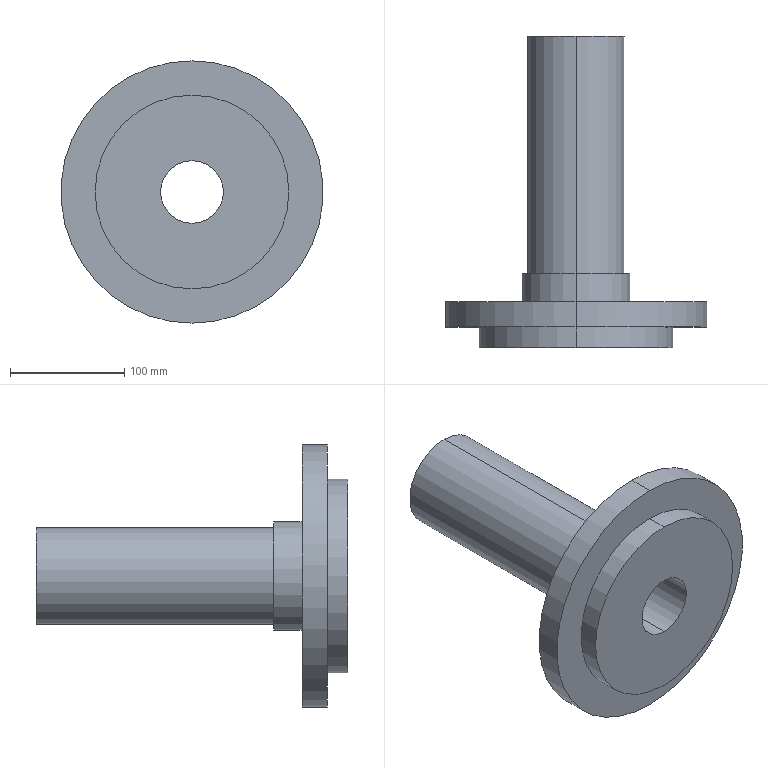Part | SolidWorks | features BaseBody 1 | 1 solid | 15 faces | box 230 x 273 x 230 mm | volume 2031428 mm3 | cylinder 10 | plane 5 | commonest cylinder face diameters 55 x2 84.997 x2 95 x2 170 x2 230 x2
STEP:
#1=CARTESIAN_POINT('',(0.,255.,27.5));
#2=VERTEX_POINT('',#1);
#3=CARTESIAN_POINT('',(0.,255.,-27.5));
#4=VERTEX_POINT('',#3);
#5=CARTESIAN_POINT('',(0.,255.,0.));
#6=DIRECTION('',(0.,-1.,0.));
#7=DIRECTION('',(0.,0.,-1.));
#8=AXIS2_PLACEMENT_3D('',#5,#6,#7);
#9=CIRCLE('',#8,27.5);
#10=EDGE_CURVE('',#2,#4,#9,.T.);
#11=ORIENTED_EDGE('',*,*,#10,.F.);
#12=CARTESIAN_POINT('',(0.,-18.,27.5));
#13=VERTEX_POINT('',#12);
#14=CARTESIAN_POINT('',(0.,255.,27.5));
#15=DIRECTION('',(0.,-1.,0.));
#16=VECTOR('',#15,1000.);
#17=LINE('',#14,#16);
#18=EDGE_CURVE('',#2,#13,#17,.T.);
#19=ORIENTED_EDGE('',*,*,#18,.T.);
#20=CARTESIAN_POINT('',(0.,-18.,-27.5));
#21=VERTEX_POINT('',#20);
#22=CARTESIAN_POINT('',(0.,-18.,0.));
#23=DIRECTION('',(0.,-1.,0.));
#24=DIRECTION('',(0.,0.,-1.));
#25=AXIS2_PLACEMENT_3D('',#22,#23,#24);
#26=CIRCLE('',#25,27.5);
#27=EDGE_CURVE('',#13,#21,#26,.T.);
#28=ORIENTED_EDGE('',*,*,#27,.T.);
#29=CARTESIAN_POINT('',(0.,255.,-27.5));
#30=DIRECTION('',(0.,-1.,0.));
#31=VECTOR('',#30,1000.);
#32=LINE('',#29,#31);
#33=EDGE_CURVE('',#4,#21,#32,.T.);
#34=ORIENTED_EDGE('',*,*,#33,.F.);
#35=EDGE_LOOP('',(#11,#19,#28,#34));
#36=FACE_OUTER_BOUND('',#35,.T.);
#37=CARTESIAN_POINT('',(0.,255.,0.));
#38=DIRECTION('',(0.,-1.,0.));
#39=DIRECTION('',(0.,0.,-1.));
#40=AXIS2_PLACEMENT_3D('',#37,#38,#39);
#41=CYLINDRICAL_SURFACE('',#40,27.5);
#42=ADVANCED_FACE('',(#36),#41,.F.);
#43=CARTESIAN_POINT('',(0.,255.,42.498));
#44=VERTEX_POINT('',#43);
#45=CARTESIAN_POINT('',(0.,255.,-42.498));
#46=VERTEX_POINT('',#45);
#47=CARTESIAN_POINT('',(0.,255.,0.));
#48=DIRECTION('',(0.,1.,0.));
#49=DIRECTION('',(0.,0.,1.));
#50=AXIS2_PLACEMENT_3D('',#47,#48,#49);
#51=CIRCLE('',#50,42.498);
#52=EDGE_CURVE('',#44,#46,#51,.T.);
#53=ORIENTED_EDGE('',*,*,#52,.F.);
#54=CARTESIAN_POINT('',(0.,47.,42.498));
#55=VERTEX_POINT('',#54);
#56=CARTESIAN_POINT('',(0.,255.,42.498));
#57=DIRECTION('',(0.,-1.,0.));
#58=VECTOR('',#57,1000.);
#59=LINE('',#56,#58);
#60=EDGE_CURVE('',#44,#55,#59,.T.);
#61=ORIENTED_EDGE('',*,*,#60,.T.);
#62=CARTESIAN_POINT('',(0.,47.,-42.498));
#63=VERTEX_POINT('',#62);
#64=CARTESIAN_POINT('',(0.,47.,0.));
#65=DIRECTION('',(0.,1.,0.));
#66=DIRECTION('',(0.,0.,1.));
#67=AXIS2_PLACEMENT_3D('',#64,#65,#66);
#68=CIRCLE('',#67,42.498);
#69=EDGE_CURVE('',#55,#63,#68,.T.);
#70=ORIENTED_EDGE('',*,*,#69,.T.);
#71=CARTESIAN_POINT('',(0.,255.,-42.498));
#72=DIRECTION('',(0.,-1.,0.));
#73=VECTOR('',#72,1000.);
#74=LINE('',#71,#73);
#75=EDGE_CURVE('',#46,#63,#74,.T.);
#76=ORIENTED_EDGE('',*,*,#75,.F.);
#77=EDGE_LOOP('',(#53,#61,#70,#76));
#78=FACE_OUTER_BOUND('',#77,.T.);
#79=CARTESIAN_POINT('',(0.,255.,0.));
#80=DIRECTION('',(0.,-1.,0.));
#81=DIRECTION('',(0.,0.,-1.));
#82=AXIS2_PLACEMENT_3D('',#79,#80,#81);
#83=CYLINDRICAL_SURFACE('',#82,42.498);
#84=ADVANCED_FACE('',(#78),#83,.T.);
#85=CARTESIAN_POINT('',(0.,47.,47.5));
#86=VERTEX_POINT('',#85);
#87=CARTESIAN_POINT('',(0.,47.,-47.5));
#88=VERTEX_POINT('',#87);
#89=CARTESIAN_POINT('',(0.,47.,0.));
#90=DIRECTION('',(0.,1.,0.));
#91=DIRECTION('',(0.,0.,1.));
#92=AXIS2_PLACEMENT_3D('',#89,#90,#91);
#93=CIRCLE('',#92,47.5);
#94=EDGE_CURVE('',#86,#88,#93,.T.);
#95=ORIENTED_EDGE('',*,*,#94,.F.);
#96=CARTESIAN_POINT('',(0.,22.,47.5));
#97=VERTEX_POINT('',#96);
#98=CARTESIAN_POINT('',(0.,47.,47.5));
#99=DIRECTION('',(0.,-1.,0.));
#100=VECTOR('',#99,1000.);
#101=LINE('',#98,#100);
#102=EDGE_CURVE('',#86,#97,#101,.T.);
#103=ORIENTED_EDGE('',*,*,#102,.T.);
#104=CARTESIAN_POINT('',(0.,22.,-47.5));
#105=VERTEX_POINT('',#104);
#106=CARTESIAN_POINT('',(0.,22.,0.));
#107=DIRECTION('',(0.,1.,0.));
#108=DIRECTION('',(0.,0.,1.));
#109=AXIS2_PLACEMENT_3D('',#106,#107,#108);
#110=CIRCLE('',#109,47.5);
#111=EDGE_CURVE('',#97,#105,#110,.T.);
#112=ORIENTED_EDGE('',*,*,#111,.T.);
#113=CARTESIAN_POINT('',(0.,47.,-47.5));
#114=DIRECTION('',(0.,-1.,0.));
#115=VECTOR('',#114,1000.);
#116=LINE('',#113,#115);
#117=EDGE_CURVE('',#88,#105,#116,.T.);
#118=ORIENTED_EDGE('',*,*,#117,.F.);
#119=EDGE_LOOP('',(#95,#103,#112,#118));
#120=FACE_OUTER_BOUND('',#119,.T.);
#121=CARTESIAN_POINT('',(0.,47.,0.));
#122=DIRECTION('',(0.,-1.,0.));
#123=DIRECTION('',(0.,0.,-1.));
#124=AXIS2_PLACEMENT_3D('',#121,#122,#123);
#125=CYLINDRICAL_SURFACE('',#124,47.5);
#126=ADVANCED_FACE('',(#120),#125,.T.);
#127=CARTESIAN_POINT('',(0.,-18.,-85.));
#128=VERTEX_POINT('',#127);
#129=CARTESIAN_POINT('',(0.,-18.,85.));
#130=VERTEX_POINT('',#129);
#131=CARTESIAN_POINT('',(0.,-18.,0.));
#132=DIRECTION('',(0.,-1.,0.));
#133=DIRECTION('',(0.,0.,-1.));
#134=AXIS2_PLACEMENT_3D('',#131,#132,#133);
#135=CIRCLE('',#134,85.);
#136=EDGE_CURVE('',#128,#130,#135,.T.);
#137=ORIENTED_EDGE('',*,*,#136,.F.);
#138=CARTESIAN_POINT('',(0.,0.,-85.));
#139=VERTEX_POINT('',#138);
#140=CARTESIAN_POINT('',(0.,-18.,-85.));
#141=DIRECTION('',(0.,1.,0.));
#142=VECTOR('',#141,1000.);
#143=LINE('',#140,#142);
#144=EDGE_CURVE('',#128,#139,#143,.T.);
#145=ORIENTED_EDGE('',*,*,#144,.T.);
#146=CARTESIAN_POINT('',(0.,0.,85.));
#147=VERTEX_POINT('',#146);
#148=CARTESIAN_POINT('',(0.,0.,0.));
#149=DIRECTION('',(0.,-1.,0.));
#150=DIRECTION('',(0.,0.,-1.));
#151=AXIS2_PLACEMENT_3D('',#148,#149,#150);
#152=CIRCLE('',#151,85.);
#153=EDGE_CURVE('',#139,#147,#152,.T.);
#154=ORIENTED_EDGE('',*,*,#153,.T.);
#155=CARTESIAN_POINT('',(0.,-18.,85.));
#156=DIRECTION('',(0.,1.,0.));
#157=VECTOR('',#156,1000.);
#158=LINE('',#155,#157);
#159=EDGE_CURVE('',#130,#147,#158,.T.);
#160=ORIENTED_EDGE('',*,*,#159,.F.);
#161=EDGE_LOOP('',(#137,#145,#154,#160));
#162=FACE_OUTER_BOUND('',#161,.T.);
#163=CARTESIAN_POINT('',(0.,-18.,0.));
#164=DIRECTION('',(0.,1.,0.));
#165=DIRECTION('',(0.,0.,1.));
#166=AXIS2_PLACEMENT_3D('',#163,#164,#165);
#167=CYLINDRICAL_SURFACE('',#166,85.);
#168=ADVANCED_FACE('',(#162),#167,.T.);
#169=CARTESIAN_POINT('',(0.,22.,115.));
#170=VERTEX_POINT('',#169);
#171=CARTESIAN_POINT('',(0.,22.,-115.));
#172=VERTEX_POINT('',#171);
#173=CARTESIAN_POINT('',(0.,22.,0.));
#174=DIRECTION('',(0.,1.,0.));
#175=DIRECTION('',(0.,0.,1.));
#176=AXIS2_PLACEMENT_3D('',#173,#174,#175);
#177=CIRCLE('',#176,115.);
#178=EDGE_CURVE('',#170,#172,#177,.T.);
#179=ORIENTED_EDGE('',*,*,#178,.F.);
#180=CARTESIAN_POINT('',(0.,0.,115.));
#181=VERTEX_POINT('',#180);
#182=CARTESIAN_POINT('',(0.,22.,115.));
#183=DIRECTION('',(0.,-1.,0.));
#184=VECTOR('',#183,1000.);
#185=LINE('',#182,#184);
#186=EDGE_CURVE('',#170,#181,#185,.T.);
#187=ORIENTED_EDGE('',*,*,#186,.T.);
#188=CARTESIAN_POINT('',(0.,0.,-115.));
#189=VERTEX_POINT('',#188);
#190=CARTESIAN_POINT('',(0.,0.,0.));
#191=DIRECTION('',(0.,1.,0.));
#192=DIRECTION('',(0.,0.,1.));
#193=AXIS2_PLACEMENT_3D('',#190,#191,#192);
#194=CIRCLE('',#193,115.);
#195=EDGE_CURVE('',#181,#189,#194,.T.);
#196=ORIENTED_EDGE('',*,*,#195,.T.);
#197=CARTESIAN_POINT('',(0.,22.,-115.));
#198=DIRECTION('',(0.,-1.,0.));
#199=VECTOR('',#198,1000.);
#200=LINE('',#197,#199);
#201=EDGE_CURVE('',#172,#189,#200,.T.);
#202=ORIENTED_EDGE('',*,*,#201,.F.);
#203=EDGE_LOOP('',(#179,#187,#196,#202));
#204=FACE_OUTER_BOUND('',#203,.T.);
#205=CARTESIAN_POINT('',(0.,22.,0.));
#206=DIRECTION('',(0.,-1.,0.));
#207=DIRECTION('',(0.,0.,-1.));
#208=AXIS2_PLACEMENT_3D('',#205,#206,#207);
#209=CYLINDRICAL_SURFACE('',#208,115.);
#210=ADVANCED_FACE('',(#204),#209,.T.);
#211=ORIENTED_EDGE('',*,*,#186,.F.);
#212=CARTESIAN_POINT('',(0.,22.,0.));
#213=DIRECTION('',(0.,1.,0.));
#214=DIRECTION('',(0.,0.,1.));
#215=AXIS2_PLACEMENT_3D('',#212,#213,#214);
#216=CIRCLE('',#215,115.);
#217=EDGE_CURVE('',#172,#170,#216,.T.);
#218=ORIENTED_EDGE('',*,*,#217,.F.);
#219=ORIENTED_EDGE('',*,*,#201,.T.);
#220=CARTESIAN_POINT('',(0.,0.,0.));
#221=DIRECTION('',(0.,1.,0.));
#222=DIRECTION('',(0.,0.,1.));
#223=AXIS2_PLACEMENT_3D('',#220,#221,#222);
#224=CIRCLE('',#223,115.);
#225=EDGE_CURVE('',#189,#181,#224,.T.);
#226=ORIENTED_EDGE('',*,*,#225,.T.);
#227=EDGE_LOOP('',(#211,#218,#219,#226));
#228=FACE_OUTER_BOUND('',#227,.T.);
#229=CARTESIAN_POINT('',(0.,22.,0.));
#230=DIRECTION('',(0.,-1.,0.));
#231=DIRECTION('',(0.,0.,-1.));
#232=AXIS2_PLACEMENT_3D('',#229,#230,#231);
#233=CYLINDRICAL_SURFACE('',#232,115.);
#234=ADVANCED_FACE('',(#228),#233,.T.);
#235=CARTESIAN_POINT('',(0.,22.,0.));
#236=DIRECTION('',(0.,1.,0.));
#237=DIRECTION('',(0.,0.,1.));
#238=AXIS2_PLACEMENT_3D('',#235,#236,#237);
#239=CIRCLE('',#238,47.5);
#240=EDGE_CURVE('',#105,#97,#239,.T.);
#241=ORIENTED_EDGE('',*,*,#240,.F.);
#242=ORIENTED_EDGE('',*,*,#111,.F.);
#243=EDGE_LOOP('',(#241,#242));
#244=FACE_BOUND('',#243,.T.);
#245=ORIENTED_EDGE('',*,*,#217,.T.);
#246=ORIENTED_EDGE('',*,*,#178,.T.);
#247=EDGE_LOOP('',(#245,#246));
#248=FACE_OUTER_BOUND('',#247,.T.);
#249=CARTESIAN_POINT('',(0.,22.,0.));
#250=DIRECTION('',(0.,1.,0.));
#251=DIRECTION('',(0.,0.,1.));
#252=AXIS2_PLACEMENT_3D('',#249,#250,#251);
#253=PLANE('',#252);
#254=ADVANCED_FACE('',(#244,#248),#253,.T.);
#255=CARTESIAN_POINT('',(0.,0.,0.));
#256=DIRECTION('',(0.,-1.,0.));
#257=DIRECTION('',(0.,0.,-1.));
#258=AXIS2_PLACEMENT_3D('',#255,#256,#257);
#259=CIRCLE('',#258,85.);
#260=EDGE_CURVE('',#147,#139,#259,.T.);
#261=ORIENTED_EDGE('',*,*,#260,.F.);
#262=ORIENTED_EDGE('',*,*,#153,.F.);
#263=EDGE_LOOP('',(#261,#262));
#264=FACE_BOUND('',#263,.T.);
#265=ORIENTED_EDGE('',*,*,#225,.F.);
#266=ORIENTED_EDGE('',*,*,#195,.F.);
#267=EDGE_LOOP('',(#265,#266));
#268=FACE_OUTER_BOUND('',#267,.T.);
#269=CARTESIAN_POINT('',(0.,0.,0.));
#270=DIRECTION('',(0.,1.,0.));
#271=DIRECTION('',(0.,0.,1.));
#272=AXIS2_PLACEMENT_3D('',#269,#270,#271);
#273=PLANE('',#272);
#274=ADVANCED_FACE('',(#264,#268),#273,.F.);
#275=ORIENTED_EDGE('',*,*,#144,.F.);
#276=CARTESIAN_POINT('',(0.,-18.,0.));
#277=DIRECTION('',(0.,-1.,0.));
#278=DIRECTION('',(0.,0.,-1.));
#279=AXIS2_PLACEMENT_3D('',#276,#277,#278);
#280=CIRCLE('',#279,85.);
#281=EDGE_CURVE('',#130,#128,#280,.T.);
#282=ORIENTED_EDGE('',*,*,#281,.F.);
#283=ORIENTED_EDGE('',*,*,#159,.T.);
#284=ORIENTED_EDGE('',*,*,#260,.T.);
#285=EDGE_LOOP('',(#275,#282,#283,#284));
#286=FACE_OUTER_BOUND('',#285,.T.);
#287=CARTESIAN_POINT('',(0.,-18.,0.));
#288=DIRECTION('',(0.,1.,0.));
#289=DIRECTION('',(0.,0.,1.));
#290=AXIS2_PLACEMENT_3D('',#287,#288,#289);
#291=CYLINDRICAL_SURFACE('',#290,85.);
#292=ADVANCED_FACE('',(#286),#291,.T.);
#293=CARTESIAN_POINT('',(0.,-18.,0.));
#294=DIRECTION('',(0.,-1.,0.));
#295=DIRECTION('',(0.,0.,-1.));
#296=AXIS2_PLACEMENT_3D('',#293,#294,#295);
#297=CIRCLE('',#296,27.5);
#298=EDGE_CURVE('',#21,#13,#297,.T.);
#299=ORIENTED_EDGE('',*,*,#298,.F.);
#300=ORIENTED_EDGE('',*,*,#27,.F.);
#301=EDGE_LOOP('',(#299,#300));
#302=FACE_BOUND('',#301,.T.);
#303=ORIENTED_EDGE('',*,*,#281,.T.);
#304=ORIENTED_EDGE('',*,*,#136,.T.);
#305=EDGE_LOOP('',(#303,#304));
#306=FACE_OUTER_BOUND('',#305,.T.);
#307=CARTESIAN_POINT('',(0.,-18.,0.));
#308=DIRECTION('',(0.,-1.,0.));
#309=DIRECTION('',(0.,0.,-1.));
#310=AXIS2_PLACEMENT_3D('',#307,#308,#309);
#311=PLANE('',#310);
#312=ADVANCED_FACE('',(#302,#306),#311,.T.);
#313=ORIENTED_EDGE('',*,*,#102,.F.);
#314=CARTESIAN_POINT('',(0.,47.,0.));
#315=DIRECTION('',(0.,1.,0.));
#316=DIRECTION('',(0.,0.,1.));
#317=AXIS2_PLACEMENT_3D('',#314,#315,#316);
#318=CIRCLE('',#317,47.5);
#319=EDGE_CURVE('',#88,#86,#318,.T.);
#320=ORIENTED_EDGE('',*,*,#319,.F.);
#321=ORIENTED_EDGE('',*,*,#117,.T.);
#322=ORIENTED_EDGE('',*,*,#240,.T.);
#323=EDGE_LOOP('',(#313,#320,#321,#322));
#324=FACE_OUTER_BOUND('',#323,.T.);
#325=CARTESIAN_POINT('',(0.,47.,0.));
#326=DIRECTION('',(0.,-1.,0.));
#327=DIRECTION('',(0.,0.,-1.));
#328=AXIS2_PLACEMENT_3D('',#325,#326,#327);
#329=CYLINDRICAL_SURFACE('',#328,47.5);
#330=ADVANCED_FACE('',(#324),#329,.T.);
#331=CARTESIAN_POINT('',(0.,47.,0.));
#332=DIRECTION('',(0.,1.,0.));
#333=DIRECTION('',(0.,0.,1.));
#334=AXIS2_PLACEMENT_3D('',#331,#332,#333);
#335=CIRCLE('',#334,42.498);
#336=EDGE_CURVE('',#63,#55,#335,.T.);
#337=ORIENTED_EDGE('',*,*,#336,.F.);
#338=ORIENTED_EDGE('',*,*,#69,.F.);
#339=EDGE_LOOP('',(#337,#338));
#340=FACE_BOUND('',#339,.T.);
#341=ORIENTED_EDGE('',*,*,#319,.T.);
#342=ORIENTED_EDGE('',*,*,#94,.T.);
#343=EDGE_LOOP('',(#341,#342));
#344=FACE_OUTER_BOUND('',#343,.T.);
#345=CARTESIAN_POINT('',(0.,47.,0.));
#346=DIRECTION('',(0.,1.,0.));
#347=DIRECTION('',(0.,0.,1.));
#348=AXIS2_PLACEMENT_3D('',#345,#346,#347);
#349=PLANE('',#348);
#350=ADVANCED_FACE('',(#340,#344),#349,.T.);
#351=ORIENTED_EDGE('',*,*,#60,.F.);
#352=CARTESIAN_POINT('',(0.,255.,0.));
#353=DIRECTION('',(0.,1.,0.));
#354=DIRECTION('',(0.,0.,1.));
#355=AXIS2_PLACEMENT_3D('',#352,#353,#354);
#356=CIRCLE('',#355,42.498);
#357=EDGE_CURVE('',#46,#44,#356,.T.);
#358=ORIENTED_EDGE('',*,*,#357,.F.);
#359=ORIENTED_EDGE('',*,*,#75,.T.);
#360=ORIENTED_EDGE('',*,*,#336,.T.);
#361=EDGE_LOOP('',(#351,#358,#359,#360));
#362=FACE_OUTER_BOUND('',#361,.T.);
#363=CARTESIAN_POINT('',(0.,255.,0.));
#364=DIRECTION('',(0.,-1.,0.));
#365=DIRECTION('',(0.,0.,-1.));
#366=AXIS2_PLACEMENT_3D('',#363,#364,#365);
#367=CYLINDRICAL_SURFACE('',#366,42.498);
#368=ADVANCED_FACE('',(#362),#367,.T.);
#369=CARTESIAN_POINT('',(0.,255.,0.));
#370=DIRECTION('',(0.,-1.,0.));
#371=DIRECTION('',(0.,0.,-1.));
#372=AXIS2_PLACEMENT_3D('',#369,#370,#371);
#373=CIRCLE('',#372,27.5);
#374=EDGE_CURVE('',#4,#2,#373,.T.);
#375=ORIENTED_EDGE('',*,*,#374,.T.);
#376=ORIENTED_EDGE('',*,*,#10,.T.);
#377=EDGE_LOOP('',(#375,#376));
#378=FACE_BOUND('',#377,.T.);
#379=ORIENTED_EDGE('',*,*,#357,.T.);
#380=ORIENTED_EDGE('',*,*,#52,.T.);
#381=EDGE_LOOP('',(#379,#380));
#382=FACE_OUTER_BOUND('',#381,.T.);
#383=CARTESIAN_POINT('',(0.,255.,0.));
#384=DIRECTION('',(0.,1.,0.));
#385=DIRECTION('',(0.,0.,1.));
#386=AXIS2_PLACEMENT_3D('',#383,#384,#385);
#387=PLANE('',#386);
#388=ADVANCED_FACE('',(#378,#382),#387,.T.);
#389=ORIENTED_EDGE('',*,*,#18,.F.);
#390=ORIENTED_EDGE('',*,*,#374,.F.);
#391=ORIENTED_EDGE('',*,*,#33,.T.);
#392=ORIENTED_EDGE('',*,*,#298,.T.);
#393=EDGE_LOOP('',(#389,#390,#391,#392));
#394=FACE_OUTER_BOUND('',#393,.T.);
#395=CARTESIAN_POINT('',(0.,255.,0.));
#396=DIRECTION('',(0.,-1.,0.));
#397=DIRECTION('',(0.,0.,-1.));
#398=AXIS2_PLACEMENT_3D('',#395,#396,#397);
#399=CYLINDRICAL_SURFACE('',#398,27.5);
#400=ADVANCED_FACE('',(#394),#399,.F.);
#401=CLOSED_SHELL('',(#42,#84,#126,#168,#210,#234,#254,#274,#292,#312,#330,#350,#368,#388,#400));
#402=MANIFOLD_SOLID_BREP('',#401);
#403=CARTESIAN_POINT('',(0.,0.,0.));
#404=DIRECTION('',(0.,0.,1.));
#405=DIRECTION('',(1.,0.,0.));
#406=AXIS2_PLACEMENT_3D('',#403,#404,#405);
#407=(LENGTH_UNIT()NAMED_UNIT(*)SI_UNIT(.MILLI.,.METRE.));
#408=UNCERTAINTY_MEASURE_WITH_UNIT(LENGTH_MEASURE(0.00001),#407,'','');
#409=(NAMED_UNIT(*)PLANE_ANGLE_UNIT()SI_UNIT($,.RADIAN.));
#410=(NAMED_UNIT(*)SI_UNIT($,.STERADIAN.)SOLID_ANGLE_UNIT());
#411=(GEOMETRIC_REPRESENTATION_CONTEXT(3)GLOBAL_UNCERTAINTY_ASSIGNED_CONTEXT((#408))GLOBAL_UNIT_ASSIGNED_CONTEXT((#407,#409,#410))REPRESENTATION_CONTEXT('',''));
#412=ADVANCED_BREP_SHAPE_REPRESENTATION('',(#402,#406),#411);